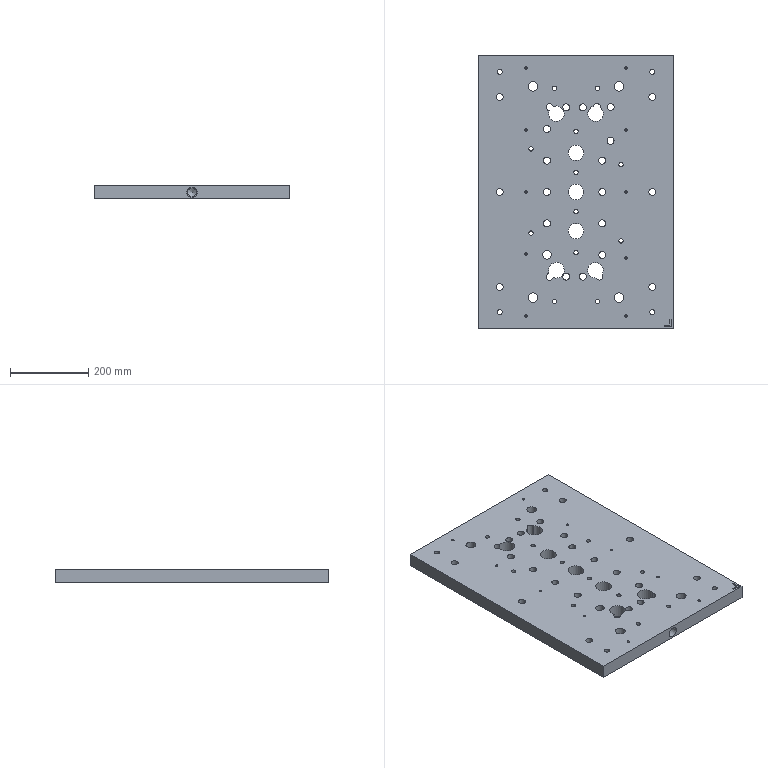Part | STEP file | BD | 1 solid | 185 faces | box 500 x 700 x 35 mm | volume 11472852 mm3 | cylinder 92 | plane 53 | cone 38 | spline 2 | commonest cylinder face diameters 18 x36 11 x12 6 x10 26 x8 40 x7 13 x4